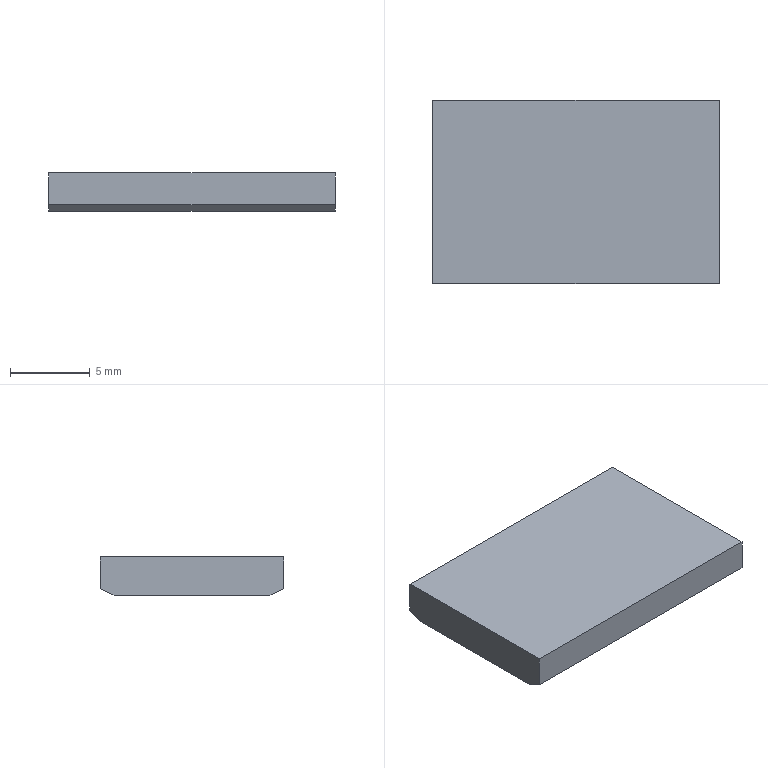Part | STEP file | CHIWA_5_1_2_1_1 | 1 solid | 8 faces | box 18 x 11.5 x 2.4 mm | volume 490.68 mm3 | plane 8
STEP:
#1=CARTESIAN_POINT('',(0.,0.,0.));
#2=DIRECTION('',(0.,0.,1.));
#3=DIRECTION('',(1.,0.,0.));
#4=AXIS2_PLACEMENT_3D('',#1,#2,#3);
#5=CARTESIAN_POINT('',(0.,4.9,-1.));
#6=VERTEX_POINT('',#5);
#7=CARTESIAN_POINT('',(0.,5.75,-0.6));
#8=VERTEX_POINT('',#7);
#9=CARTESIAN_POINT('',(0.,4.9,-1.));
#10=DIRECTION('',(0.,0.9048,0.4258));
#11=VECTOR('',#10,0.9394);
#12=LINE('',#9,#11);
#13=EDGE_CURVE('',#6,#8,#12,.T.);
#14=ORIENTED_EDGE('',*,*,#13,.T.);
#15=CARTESIAN_POINT('',(0.,5.75,1.4));
#16=VERTEX_POINT('',#15);
#17=CARTESIAN_POINT('',(0.,5.75,-0.6));
#18=DIRECTION('',(0.,0.,1.));
#19=VECTOR('',#18,2.);
#20=LINE('',#17,#19);
#21=EDGE_CURVE('',#8,#16,#20,.T.);
#22=ORIENTED_EDGE('',*,*,#21,.T.);
#23=CARTESIAN_POINT('',(0.,-5.75,1.4));
#24=VERTEX_POINT('',#23);
#25=CARTESIAN_POINT('',(0.,5.75,1.4));
#26=DIRECTION('',(0.,-1.,0.));
#27=VECTOR('',#26,11.5);
#28=LINE('',#25,#27);
#29=EDGE_CURVE('',#16,#24,#28,.T.);
#30=ORIENTED_EDGE('',*,*,#29,.T.);
#31=CARTESIAN_POINT('',(0.,-5.75,-0.6));
#32=VERTEX_POINT('',#31);
#33=CARTESIAN_POINT('',(0.,-5.75,1.4));
#34=DIRECTION('',(0.,0.,-1.));
#35=VECTOR('',#34,2.);
#36=LINE('',#33,#35);
#37=EDGE_CURVE('',#24,#32,#36,.T.);
#38=ORIENTED_EDGE('',*,*,#37,.T.);
#39=CARTESIAN_POINT('',(0.,-4.9,-1.));
#40=VERTEX_POINT('',#39);
#41=CARTESIAN_POINT('',(0.,-5.75,-0.6));
#42=DIRECTION('',(0.,0.9048,-0.4258));
#43=VECTOR('',#42,0.9394);
#44=LINE('',#41,#43);
#45=EDGE_CURVE('',#32,#40,#44,.T.);
#46=ORIENTED_EDGE('',*,*,#45,.T.);
#47=CARTESIAN_POINT('',(0.,-4.9,-1.));
#48=DIRECTION('',(0.,1.,0.));
#49=VECTOR('',#48,9.8);
#50=LINE('',#47,#49);
#51=EDGE_CURVE('',#40,#6,#50,.T.);
#52=ORIENTED_EDGE('',*,*,#51,.T.);
#53=EDGE_LOOP('',(#14,#22,#30,#38,#46,#52));
#54=FACE_OUTER_BOUND('',#53,.F.);
#55=CARTESIAN_POINT('',(0.,0.,0.));
#56=DIRECTION('',(1.,0.,0.));
#57=DIRECTION('',(0.,-1.,0.));
#58=AXIS2_PLACEMENT_3D('',#55,#56,#57);
#59=PLANE('',#58);
#60=ADVANCED_FACE('',(#54),#59,.F.);
#61=ORIENTED_EDGE('',*,*,#13,.F.);
#62=CARTESIAN_POINT('',(18.,4.9,-1.));
#63=VERTEX_POINT('',#62);
#64=CARTESIAN_POINT('',(0.,4.9,-1.));
#65=DIRECTION('',(1.,0.,0.));
#66=VECTOR('',#65,18.);
#67=LINE('',#64,#66);
#68=EDGE_CURVE('',#6,#63,#67,.T.);
#69=ORIENTED_EDGE('',*,*,#68,.T.);
#70=CARTESIAN_POINT('',(18.,5.75,-0.6));
#71=VERTEX_POINT('',#70);
#72=CARTESIAN_POINT('',(18.,5.75,-0.6));
#73=DIRECTION('',(0.,-0.9048,-0.4258));
#74=VECTOR('',#73,0.9394);
#75=LINE('',#72,#74);
#76=EDGE_CURVE('',#71,#63,#75,.T.);
#77=ORIENTED_EDGE('',*,*,#76,.F.);
#78=CARTESIAN_POINT('',(0.,5.75,-0.6));
#79=DIRECTION('',(1.,0.,0.));
#80=VECTOR('',#79,18.);
#81=LINE('',#78,#80);
#82=EDGE_CURVE('',#8,#71,#81,.T.);
#83=ORIENTED_EDGE('',*,*,#82,.F.);
#84=EDGE_LOOP('',(#61,#69,#77,#83));
#85=FACE_OUTER_BOUND('',#84,.F.);
#86=CARTESIAN_POINT('',(0.,4.9,-1.));
#87=DIRECTION('',(0.,0.4258,-0.9048));
#88=DIRECTION('',(0.,0.9048,0.4258));
#89=AXIS2_PLACEMENT_3D('',#86,#87,#88);
#90=PLANE('',#89);
#91=ADVANCED_FACE('',(#85),#90,.T.);
#92=ORIENTED_EDGE('',*,*,#51,.F.);
#93=CARTESIAN_POINT('',(18.,-4.9,-1.));
#94=VERTEX_POINT('',#93);
#95=CARTESIAN_POINT('',(0.,-4.9,-1.));
#96=DIRECTION('',(1.,0.,0.));
#97=VECTOR('',#96,18.);
#98=LINE('',#95,#97);
#99=EDGE_CURVE('',#40,#94,#98,.T.);
#100=ORIENTED_EDGE('',*,*,#99,.T.);
#101=CARTESIAN_POINT('',(18.,-4.9,-1.));
#102=DIRECTION('',(0.,1.,0.));
#103=VECTOR('',#102,9.8);
#104=LINE('',#101,#103);
#105=EDGE_CURVE('',#94,#63,#104,.T.);
#106=ORIENTED_EDGE('',*,*,#105,.T.);
#107=ORIENTED_EDGE('',*,*,#68,.F.);
#108=EDGE_LOOP('',(#92,#100,#106,#107));
#109=FACE_OUTER_BOUND('',#108,.F.);
#110=CARTESIAN_POINT('',(0.,-4.9,-1.));
#111=DIRECTION('',(0.,0.,-1.));
#112=DIRECTION('',(0.,1.,0.));
#113=AXIS2_PLACEMENT_3D('',#110,#111,#112);
#114=PLANE('',#113);
#115=ADVANCED_FACE('',(#109),#114,.T.);
#116=ORIENTED_EDGE('',*,*,#45,.F.);
#117=CARTESIAN_POINT('',(18.,-5.75,-0.6));
#118=VERTEX_POINT('',#117);
#119=CARTESIAN_POINT('',(0.,-5.75,-0.6));
#120=DIRECTION('',(1.,0.,0.));
#121=VECTOR('',#120,18.);
#122=LINE('',#119,#121);
#123=EDGE_CURVE('',#32,#118,#122,.T.);
#124=ORIENTED_EDGE('',*,*,#123,.T.);
#125=CARTESIAN_POINT('',(18.,-4.9,-1.));
#126=DIRECTION('',(0.,-0.9048,0.4258));
#127=VECTOR('',#126,0.9394);
#128=LINE('',#125,#127);
#129=EDGE_CURVE('',#94,#118,#128,.T.);
#130=ORIENTED_EDGE('',*,*,#129,.F.);
#131=ORIENTED_EDGE('',*,*,#99,.F.);
#132=EDGE_LOOP('',(#116,#124,#130,#131));
#133=FACE_OUTER_BOUND('',#132,.F.);
#134=CARTESIAN_POINT('',(0.,-5.75,-0.6));
#135=DIRECTION('',(0.,-0.4258,-0.9048));
#136=DIRECTION('',(0.,0.9048,-0.4258));
#137=AXIS2_PLACEMENT_3D('',#134,#135,#136);
#138=PLANE('',#137);
#139=ADVANCED_FACE('',(#133),#138,.T.);
#140=ORIENTED_EDGE('',*,*,#37,.F.);
#141=CARTESIAN_POINT('',(18.,-5.75,1.4));
#142=VERTEX_POINT('',#141);
#143=CARTESIAN_POINT('',(0.,-5.75,1.4));
#144=DIRECTION('',(1.,0.,0.));
#145=VECTOR('',#144,18.);
#146=LINE('',#143,#145);
#147=EDGE_CURVE('',#24,#142,#146,.T.);
#148=ORIENTED_EDGE('',*,*,#147,.T.);
#149=CARTESIAN_POINT('',(18.,-5.75,1.4));
#150=DIRECTION('',(0.,0.,-1.));
#151=VECTOR('',#150,2.);
#152=LINE('',#149,#151);
#153=EDGE_CURVE('',#142,#118,#152,.T.);
#154=ORIENTED_EDGE('',*,*,#153,.T.);
#155=ORIENTED_EDGE('',*,*,#123,.F.);
#156=EDGE_LOOP('',(#140,#148,#154,#155));
#157=FACE_OUTER_BOUND('',#156,.F.);
#158=CARTESIAN_POINT('',(0.,-5.75,1.4));
#159=DIRECTION('',(0.,-1.,0.));
#160=DIRECTION('',(0.,0.,-1.));
#161=AXIS2_PLACEMENT_3D('',#158,#159,#160);
#162=PLANE('',#161);
#163=ADVANCED_FACE('',(#157),#162,.T.);
#164=ORIENTED_EDGE('',*,*,#29,.F.);
#165=CARTESIAN_POINT('',(18.,5.75,1.4));
#166=VERTEX_POINT('',#165);
#167=CARTESIAN_POINT('',(0.,5.75,1.4));
#168=DIRECTION('',(1.,0.,0.));
#169=VECTOR('',#168,18.);
#170=LINE('',#167,#169);
#171=EDGE_CURVE('',#16,#166,#170,.T.);
#172=ORIENTED_EDGE('',*,*,#171,.T.);
#173=CARTESIAN_POINT('',(18.,5.75,1.4));
#174=DIRECTION('',(0.,-1.,0.));
#175=VECTOR('',#174,11.5);
#176=LINE('',#173,#175);
#177=EDGE_CURVE('',#166,#142,#176,.T.);
#178=ORIENTED_EDGE('',*,*,#177,.T.);
#179=ORIENTED_EDGE('',*,*,#147,.F.);
#180=EDGE_LOOP('',(#164,#172,#178,#179));
#181=FACE_OUTER_BOUND('',#180,.F.);
#182=CARTESIAN_POINT('',(0.,5.75,1.4));
#183=DIRECTION('',(0.,0.,1.));
#184=DIRECTION('',(0.,-1.,0.));
#185=AXIS2_PLACEMENT_3D('',#182,#183,#184);
#186=PLANE('',#185);
#187=ADVANCED_FACE('',(#181),#186,.T.);
#188=ORIENTED_EDGE('',*,*,#21,.F.);
#189=ORIENTED_EDGE('',*,*,#82,.T.);
#190=CARTESIAN_POINT('',(18.,5.75,-0.6));
#191=DIRECTION('',(0.,0.,1.));
#192=VECTOR('',#191,2.);
#193=LINE('',#190,#192);
#194=EDGE_CURVE('',#71,#166,#193,.T.);
#195=ORIENTED_EDGE('',*,*,#194,.T.);
#196=ORIENTED_EDGE('',*,*,#171,.F.);
#197=EDGE_LOOP('',(#188,#189,#195,#196));
#198=FACE_OUTER_BOUND('',#197,.F.);
#199=CARTESIAN_POINT('',(0.,5.75,-0.6));
#200=DIRECTION('',(0.,1.,0.));
#201=DIRECTION('',(0.,0.,1.));
#202=AXIS2_PLACEMENT_3D('',#199,#200,#201);
#203=PLANE('',#202);
#204=ADVANCED_FACE('',(#198),#203,.T.);
#205=ORIENTED_EDGE('',*,*,#76,.T.);
#206=ORIENTED_EDGE('',*,*,#105,.F.);
#207=ORIENTED_EDGE('',*,*,#129,.T.);
#208=ORIENTED_EDGE('',*,*,#153,.F.);
#209=ORIENTED_EDGE('',*,*,#177,.F.);
#210=ORIENTED_EDGE('',*,*,#194,.F.);
#211=EDGE_LOOP('',(#205,#206,#207,#208,#209,#210));
#212=FACE_OUTER_BOUND('',#211,.F.);
#213=CARTESIAN_POINT('',(18.,0.,0.));
#214=DIRECTION('',(1.,0.,0.));
#215=DIRECTION('',(0.,-1.,0.));
#216=AXIS2_PLACEMENT_3D('',#213,#214,#215);
#217=PLANE('',#216);
#218=ADVANCED_FACE('',(#212),#217,.T.);
#219=CLOSED_SHELL('',(#60,#91,#115,#139,#163,#187,#204,#218));
#220=MANIFOLD_SOLID_BREP('',#219);
#221=(LENGTH_UNIT()NAMED_UNIT(*)SI_UNIT(.MILLI.,.METRE.));
#222=UNCERTAINTY_MEASURE_WITH_UNIT(LENGTH_MEASURE(0.002149),#221,'','');
#223=(NAMED_UNIT(*)PLANE_ANGLE_UNIT()SI_UNIT($,.RADIAN.));
#224=PLANE_ANGLE_MEASURE_WITH_UNIT(PLANE_ANGLE_MEASURE(0.01745),#223);
#225=(CONVERSION_BASED_UNIT('DEGREE',#224)NAMED_UNIT(*)PLANE_ANGLE_UNIT());
#226=(NAMED_UNIT(*)SI_UNIT($,.STERADIAN.)SOLID_ANGLE_UNIT());
#227=(GEOMETRIC_REPRESENTATION_CONTEXT(3)GLOBAL_UNCERTAINTY_ASSIGNED_CONTEXT((#222))GLOBAL_UNIT_ASSIGNED_CONTEXT((#221,#225,#226))REPRESENTATION_CONTEXT('',''));
#228=ADVANCED_BREP_SHAPE_REPRESENTATION('',(#4,#220),#227);